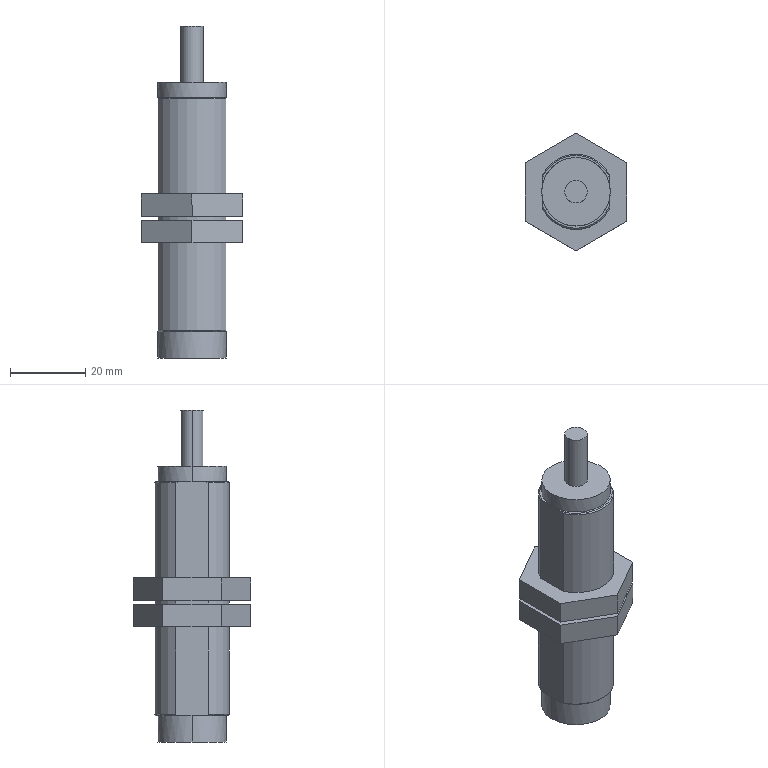Part | STEP file | Shock Absorber (SMC) RB2015 | 1 solid | 49 faces | box 27 x 31.177 x 88.2 mm | volume 26039 mm3 | plane 29 | cylinder 12 | spline 4 | cone 4 | commonest cylinder face diameters 20 x6 18.2 x4 6 x2